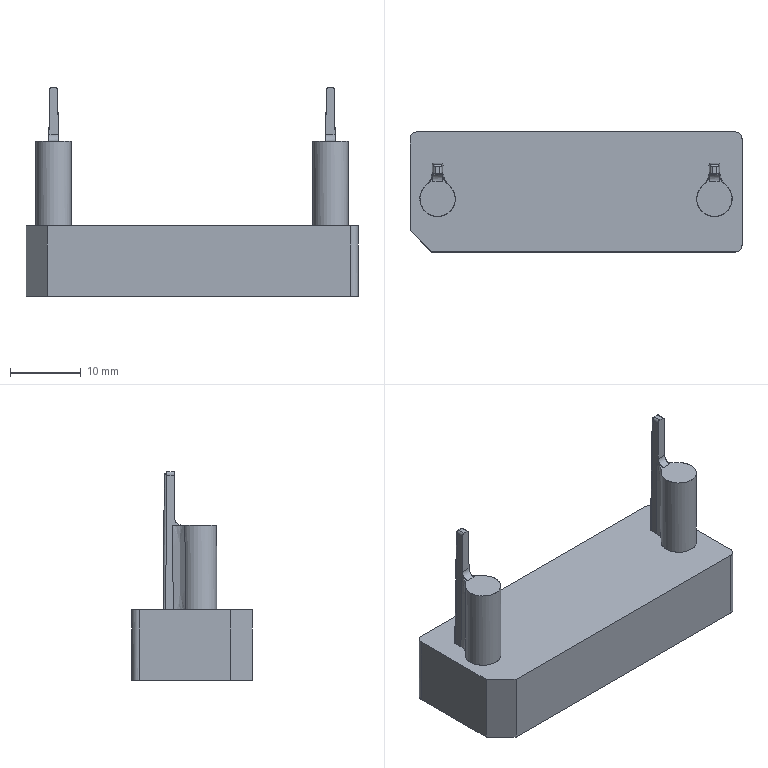NC program | PowerMill | posted with a generic post | part box 47 x 17 x 29.578 mm
Lines 293309 to 293638 of 293638:
N293406 M6
N293407 S15000 M03
N293408 G00 G90 X0.0 Y0.0
N293409 G43 Z10.298 H13
N293410
N293411 G05 P10000 R8
N293412 X-15.3323 Y7.6966
N293413 Z-19.73
N293414 G01 Z-19.83 F600.0
N293415 X-14.868 Y8.0162 F1000.0
N293416 Y5.55
N293417 G00 Z-16.6803
N293418 G01 X-13.2766 Y6.0675 F10000.0
N293419 G00 Z-19.73
N293420 G01 Z-19.83 F600.0
N293421 X-13.3263 Y6.2694 F1000.0
N293422 X-13.3561 Y6.5022
N293423 X-13.366 Y6.7662
N293424 X-13.3561 Y7.0309
N293425 X-13.3263 Y7.2645
N293426 X-13.2766 Y7.4669
N293427 X-13.2071 Y7.6382
N293428 X-13.1177 Y7.7783
N293429 X-13.0085 Y7.8873
N293430 X-12.8793 Y7.9652
N293431 X-12.7303 Y8.0119
N293432 X-12.5615 Y8.0275
N293433 X-12.3927 Y8.0119
N293434 X-12.2437 Y7.9652
N293435 X-12.1145 Y7.8873
N293436 X-12.0053 Y7.7783
N293437 X-11.9159 Y7.6382
N293438 X-11.8464 Y7.4669
N293439 X-11.7967 Y7.2645
N293440 X-11.7669 Y7.0309
N293441 X-11.757 Y6.7662
N293442 X-11.7669 Y6.5071
N293443 X-11.7967 Y6.2774
N293444 X-11.8463 Y6.0773
N293445 X-11.9157 Y5.9065
N293446 X-12.005 Y5.7652
N293447 X-12.1141 Y5.6534
N293448 X-12.2424 Y5.573
N293449 X-12.3915 Y5.5247
N293450 X-12.5615 Y5.5086
N293451 X-12.7303 Y5.5242
N293452 X-12.8793 Y5.5707
N293453 X-13.0085 Y5.6484
N293454 X-13.1177 Y5.757
N293455 X-13.2071 Y5.8968
N293456 X-13.2766 Y6.0675
N293457 G00 Z-16.6803
N293458 G01 X-9.8264 Y6.4203 F10000.0
N293459 G00 Z-19.73
N293460 G01 Z-19.83 F600.0
N293461 X-10.7719 F1000.0
N293462 G00 Z-16.6803
N293463 G01 X-6.6439 Y6.332 F10000.0
N293464 G00 Z-19.73
N293465 G01 Z-19.83 F600.0
N293466 X-6.7037 Y6.1483 F1000.0
N293467 X-6.7835 Y5.9866
N293468 X-6.8832 Y5.8466
N293469 X-7.0029 Y5.7286
N293470 X-7.1437 Y5.6324
N293471 X-7.3009 Y5.5636
N293472 X-7.4745 Y5.5224
N293473 X-7.6646 Y5.5086
N293474 X-7.8725 Y5.5215
N293475 X-8.0602 Y5.5602
N293476 X-8.2276 Y5.6247
N293477 X-8.3747 Y5.7149
N293478 X-8.5016 Y5.8309
N293479 X-8.6083 Y5.9727
N293480 X-8.6947 Y6.1402
N293481 X-8.7667 Y6.3499
N293482 X-8.81 Y6.5705
N293483 X-8.8244 Y6.8019
N293484 X-8.8128 Y7.0197
N293485 X-8.7782 Y7.2176
N293486 X-8.7204 Y7.3956
N293487 X-8.6396 Y7.5538
N293488 X-8.5357 Y7.6921
N293489 X-8.4087 Y7.8105
N293490 X-8.2586 Y7.909
N293491 X-8.071 Y7.9926
N293492 X-7.8718 Y8.0427
N293493 X-7.6608 Y8.0594
N293494 X-7.4846 Y8.0478
N293495 X-7.3225 Y8.0131
N293496 X-7.1745 Y7.9553
N293497 X-7.0405 Y7.8743
N293498 X-6.9232 Y7.7714
N293499 X-6.8248 Y7.648
N293500 X-6.7455 Y7.504
N293501 X-6.6853 Y7.3395
N293502 G00 Z-16.6803
N293503 G01 X-5.6082 Y7.2021 F10000.0
N293504 G00 Z-19.73
N293505 G01 Z-19.83 F600.0
N293506 X-5.6003 Y7.2645 F1000.0
N293507 X-5.5506 Y7.4669
N293508 X-5.4811 Y7.6382
N293509 X-5.3917 Y7.7783
N293510 X-5.2824 Y7.8873
N293511 X-5.1533 Y7.9652
N293512 X-5.0043 Y8.0119
N293513 X-4.8355 Y8.0275
N293514 X-4.6666 Y8.0119
N293515 X-4.5177 Y7.9652
N293516 X-4.3885 Y7.8873
N293517 X-4.2793 Y7.7783
N293518 X-4.1899 Y7.6382
N293519 X-4.1204 Y7.4669
N293520 X-4.0707 Y7.2645
N293521 X-4.0409 Y7.0309
N293522 X-4.031 Y6.7662
N293523 X-4.0409 Y6.5071
N293524 X-4.0707 Y6.2774
N293525 X-4.1203 Y6.0773
N293526 X-4.1897 Y5.9065
N293527 X-4.279 Y5.7652
N293528 X-4.3881 Y5.6534
N293529 X-4.5164 Y5.573
N293530 X-4.6655 Y5.5247
N293531 X-4.8355 Y5.5086
N293532 X-5.0043 Y5.5242
N293533 X-5.1533 Y5.5707
N293534 X-5.2824 Y5.6484
N293535 X-5.3917 Y5.757
N293536 X-5.4811 Y5.8968
N293537 X-5.5506 Y6.0675
N293538 X-5.6003 Y6.2694
N293539 X-5.6301 Y6.5022
N293540 X-5.64 Y6.7662
N293541 X-5.6301 Y7.0309
N293542 X-5.6082 Y7.2021
N293543 G00 Z-16.6803
N293544 G01 X-2.3241 Y7.6966 F10000.0
N293545 G00 Z-19.73
N293546 G01 Z-19.83 F600.0
N293547 X-1.8598 Y8.0162 F1000.0
N293548 Y5.55
N293549 G00 Z-16.6803
N293550 G01 X0.5408 Y6.4203 F10000.0
N293551 G00 Z-19.73
N293552 G01 Z-19.83 F600.0
N293553 X-0.4047 F1000.0
N293554 G00 Z-16.6803
N293555 G01 X2.3078 Y6.8771 F10000.0
N293556 G00 Z-19.73
N293557 G01 Z-19.83 F600.0
N293558 X2.1119 Y6.9013 F1000.0
N293559 X1.9528 Y6.9389
N293560 X1.8304 Y6.9899
N293561 X1.7342 Y7.0614
N293562 X1.6654 Y7.152
N293563 X1.6242 Y7.2616
N293564 X1.6104 Y7.3902
N293565 X1.6238 Y7.5242
N293566 X1.664 Y7.6459
N293567 X1.731 Y7.7554
N293568 X1.8247 Y7.8526
N293569 X1.9332 Y7.9291
N293570 X2.0517 Y7.9837
N293571 X2.1803 Y8.0165
N293572 X2.3191 Y8.0275
N293573 X2.4624 Y8.0168
N293574 X2.5935 Y7.9847
N293575 X2.7124 Y7.9312
N293576 X2.8191 Y7.8564
N293577 X2.9137 Y7.7591
N293578 X2.9812 Y7.6478
N293579 X3.0218 Y7.5223
N293580 X3.0353 Y7.3827
N293581 X3.0204 Y7.2555
N293582 X2.9759 Y7.1466
N293583 X2.9016 Y7.056
N293584 X2.7977 Y6.9838
N293585 X2.6641 Y6.9299
N293586 X2.5008 Y6.8943
N293587 X2.3078 Y6.8771
N293588 X2.5059 Y6.8477
N293589 X2.6678 Y6.816
N293590 X2.7935 Y6.7819
N293591 X2.883 Y6.7455
N293592 X2.9744 Y6.682
N293593 X3.0454 Y6.6011
N293594 X3.0962 Y6.503
N293595 X3.1266 Y6.3876
N293596 X3.1368 Y6.2549
N293597 X3.1218 Y6.093
N293598 X3.0771 Y5.9476
N293599 X3.0025 Y5.8186
N293600 X2.898 Y5.706
N293601 X2.7761 Y5.6197
N293602 X2.6396 Y5.558
N293603 X2.4885 Y5.521
N293604 X2.3228 Y5.5086
N293605 X2.1565 Y5.5212
N293606 X2.0052 Y5.5589
N293607 X1.8689 Y5.6218
N293608 X1.7477 Y5.7098
N293609 X1.644 Y5.8234
N293610 X1.57 Y5.9537
N293611 X1.5256 Y6.1006
N293612 X1.5108 Y6.2643
N293613 X1.5203 Y6.396
N293614 X1.5487 Y6.51
N293615 X1.5961 Y6.6062
N293616 X1.6624 Y6.6847
N293617 X1.7477 Y6.7455
N293618 X1.8299 Y6.7798
N293619 X1.9507 Y6.8132
N293620 X2.11 Y6.8456
N293621 X2.3078 Y6.8771
N293622 G00 Z-16.6803
N293623 G01 X5.0542 Y6.4203 F10000.0
N293624 G00 Z-19.73
N293625 G01 Z-19.83 F600.0
N293626 X4.1087 F1000.0
N293627 G00 Z-16.6803
N293628 G01 X6.038 Y6.5022 F10000.0
N293629 G00 Z-19.73
N293630 G01 Z-19.83 F600.0
N293631 X6.028 Y6.7662 F1000.0
N293632 X6.038 Y7.0309
N293633 X6.0678 Y7.2645
N293634 X6.1174 Y7.4669
N293635 X6.1869 Y7.6382
N293636 X6.2763 Y7.7783
N293637 X6.3856 Y7.8873
N293638 X6.5147 Y7.9652
N293639 X6.6637 Y8.0119
N293640 X6.8326 Y8.0275
N293641 X7.0014 Y8.0119
N293642 X7.1504 Y7.9652
N293643 X7.2795 Y7.8873
N293644 X7.3888 Y7.7783
N293645 X7.4781 Y7.6382
N293646 X7.5477 Y7.4669
N293647 X7.5973 Y7.2645
N293648 X7.6271 Y7.0309
N293649 X7.6371 Y6.7662
N293650 X7.6271 Y6.5071
N293651 X7.5974 Y6.2774
N293652 X7.5478 Y6.0773
N293653 X7.4783 Y5.9065
N293654 X7.389 Y5.7652
N293655 X7.2799 Y5.6534
N293656 X7.1517 Y5.573
N293657 X7.0026 Y5.5247
N293658 X6.8326 Y5.5086
N293659 X6.6637 Y5.5242
N293660 X6.5147 Y5.5707
N293661 X6.3856 Y5.6484
N293662 X6.2763 Y5.757
N293663 X6.1869 Y5.8968
N293664 X6.1174 Y6.0675
N293665 X6.0678 Y6.2694
N293666 X6.038 Y6.5022
N293667 G00 Z-16.6803
N293668 G01 X8.9906 Y5.6741 F10000.0
N293669 G00 Z-19.73
N293670 G01 Z-19.83 F600.0
N293671 Y6.0154 F1000.0
N293672 G00 Z-16.6803
N293673 G01 X10.3914 Y6.2694 F10000.0
N293674 G00 Z-19.73
N293675 G01 Z-19.83 F600.0
N293676 X10.3616 Y6.5022 F1000.0
N293677 X10.3516 Y6.7662
N293678 X10.3616 Y7.0309
N293679 X10.3914 Y7.2645
N293680 X10.441 Y7.4669
N293681 X10.5106 Y7.6382
N293682 X10.5999 Y7.7783
N293683 X10.7092 Y7.8873
N293684 X10.8383 Y7.9652
N293685 X10.9873 Y8.0119
N293686 X11.1561 Y8.0275
N293687 X11.325 Y8.0119
N293688 X11.474 Y7.9652
N293689 X11.6031 Y7.8873
N293690 X11.7124 Y7.7783
N293691 X11.8018 Y7.6382
N293692 X11.8713 Y7.4669
N293693 X11.9209 Y7.2645
N293694 X11.9507 Y7.0309
N293695 X11.9607 Y6.7662
N293696 X11.9507 Y6.5071
N293697 X11.921 Y6.2774
N293698 X11.8714 Y6.0773
N293699 X11.8019 Y5.9065
N293700 X11.7126 Y5.7652
N293701 X11.6035 Y5.6534
N293702 X11.4753 Y5.573
N293703 X11.3262 Y5.5247
N293704 X11.1561 Y5.5086
N293705 X10.9873 Y5.5242
N293706 X10.8383 Y5.5707
N293707 X10.7092 Y5.6484
N293708 X10.5999 Y5.757
N293709 X10.5106 Y5.8968
N293710 X10.441 Y6.0675
N293711 X10.3914 Y6.2694
N293712 G00 Z-16.6803
N293713 G01 X13.0116 Y7.9842 F10000.0
N293714 G00 Z-19.73
N293715 G01 Z-19.83 F600.0
N293716 X14.6074 F1000.0
N293717 X14.5609 Y7.8512
N293718 X14.4913 Y7.6977
N293719 X14.3988 Y7.5237
N293720 X14.1413 Y7.082
N293721 X13.9882 Y6.7789
N293722 X13.8643 Y6.4741
N293723 X13.7695 Y6.1677
N293724 X13.704 Y5.8597
N293725 X13.6676 Y5.55
N293726 G00 Z10.298
N293727 G05 P0
N293728 (---------------)
N293729 ( END TOOLPATH : 精公刻字01-刻字-TEXT_D4 )
N293730 (---------------)
N293731
N293732 M05
N293733 G53 Z0.0
N293734 M30
%